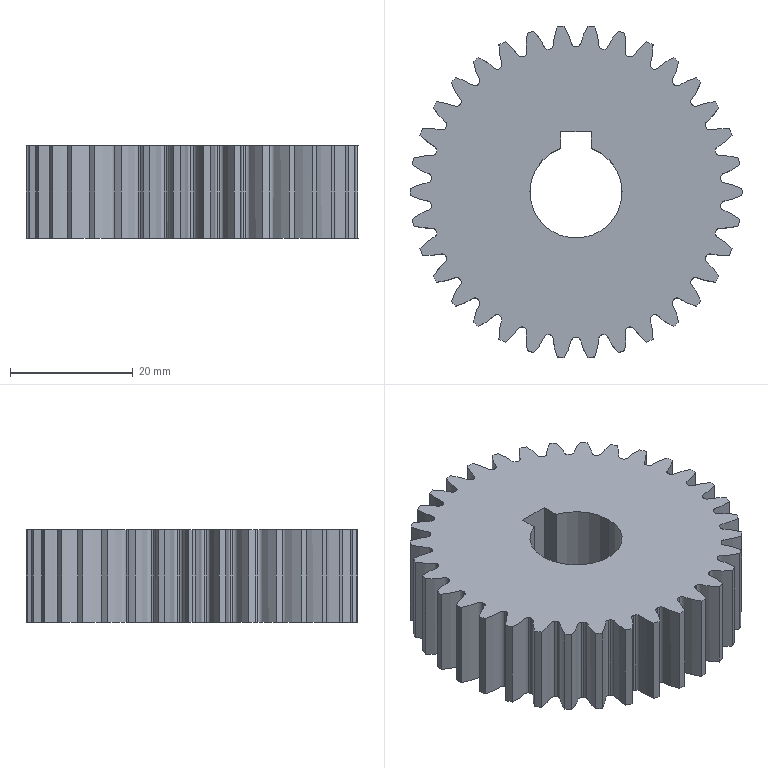Part | STEP file | 1 solid | 145 faces | box 54 x 53.862 x 15 mm | volume 27535 mm3 | cylinder 72 | spline 68 | plane 5 | commonest cylinder face diameters 54 x35 47.25 x34 15 x3